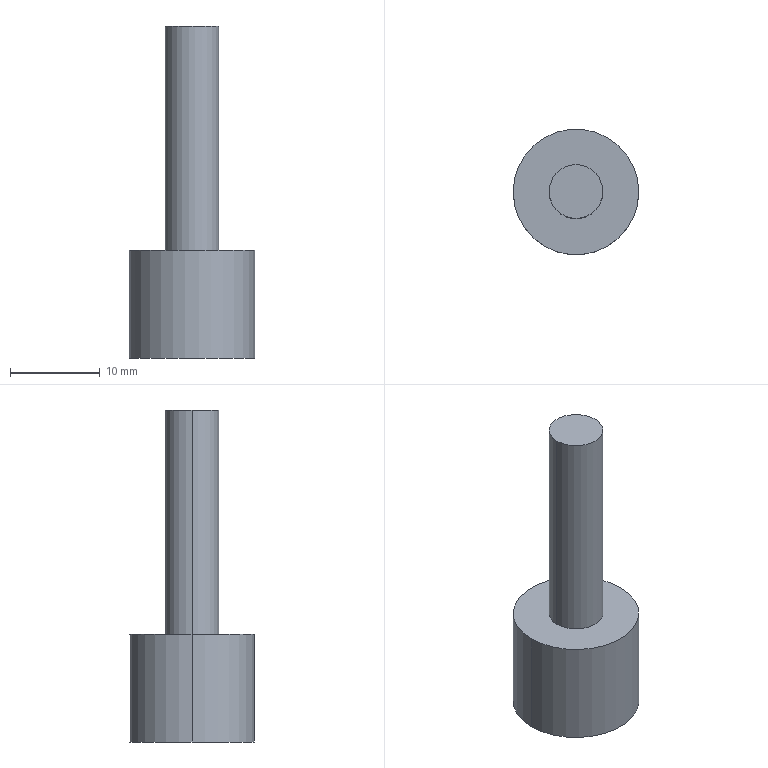Part | SolidWorks | features Extrusion 1, ICE 1 | 1 solid | 7 faces | box 14 x 14 x 37 mm | volume 2554 mm3 | cylinder 4 | plane 3 | commonest cylinder face diameters 6 x2 14 x2
STEP:
#1=CARTESIAN_POINT('',(3.,0.,37.));
#2=VERTEX_POINT('',#1);
#3=CARTESIAN_POINT('',(-3.,0.,37.));
#4=VERTEX_POINT('',#3);
#5=CARTESIAN_POINT('',(0.,0.,37.));
#6=DIRECTION('',(0.,0.,1.));
#7=DIRECTION('',(1.,0.,0.));
#8=AXIS2_PLACEMENT_3D('',#5,#6,#7);
#9=CIRCLE('',#8,3.);
#10=EDGE_CURVE('',#2,#4,#9,.T.);
#11=ORIENTED_EDGE('',*,*,#10,.F.);
#12=CARTESIAN_POINT('',(3.,0.,12.));
#13=VERTEX_POINT('',#12);
#14=CARTESIAN_POINT('',(3.,0.,37.));
#15=DIRECTION('',(0.,0.,-1.));
#16=VECTOR('',#15,1000.);
#17=LINE('',#14,#16);
#18=EDGE_CURVE('',#2,#13,#17,.T.);
#19=ORIENTED_EDGE('',*,*,#18,.T.);
#20=CARTESIAN_POINT('',(-3.,0.,12.));
#21=VERTEX_POINT('',#20);
#22=CARTESIAN_POINT('',(0.,0.,12.));
#23=DIRECTION('',(0.,0.,1.));
#24=DIRECTION('',(1.,0.,0.));
#25=AXIS2_PLACEMENT_3D('',#22,#23,#24);
#26=CIRCLE('',#25,3.);
#27=EDGE_CURVE('',#13,#21,#26,.T.);
#28=ORIENTED_EDGE('',*,*,#27,.T.);
#29=CARTESIAN_POINT('',(-3.,0.,37.));
#30=DIRECTION('',(0.,0.,-1.));
#31=VECTOR('',#30,1000.);
#32=LINE('',#29,#31);
#33=EDGE_CURVE('',#4,#21,#32,.T.);
#34=ORIENTED_EDGE('',*,*,#33,.F.);
#35=EDGE_LOOP('',(#11,#19,#28,#34));
#36=FACE_OUTER_BOUND('',#35,.T.);
#37=CARTESIAN_POINT('',(0.,0.,37.));
#38=DIRECTION('',(0.,0.,-1.));
#39=DIRECTION('',(-1.,0.,0.));
#40=AXIS2_PLACEMENT_3D('',#37,#38,#39);
#41=CYLINDRICAL_SURFACE('',#40,3.);
#42=ADVANCED_FACE('',(#36),#41,.T.);
#43=CARTESIAN_POINT('',(7.,0.,12.));
#44=VERTEX_POINT('',#43);
#45=CARTESIAN_POINT('',(-7.,0.,12.));
#46=VERTEX_POINT('',#45);
#47=CARTESIAN_POINT('',(0.,0.,12.));
#48=DIRECTION('',(0.,0.,1.));
#49=DIRECTION('',(1.,0.,0.));
#50=AXIS2_PLACEMENT_3D('',#47,#48,#49);
#51=CIRCLE('',#50,7.);
#52=EDGE_CURVE('',#44,#46,#51,.T.);
#53=ORIENTED_EDGE('',*,*,#52,.F.);
#54=CARTESIAN_POINT('',(7.,0.,0.));
#55=VERTEX_POINT('',#54);
#56=CARTESIAN_POINT('',(7.,0.,12.));
#57=DIRECTION('',(0.,0.,-1.));
#58=VECTOR('',#57,1000.);
#59=LINE('',#56,#58);
#60=EDGE_CURVE('',#44,#55,#59,.T.);
#61=ORIENTED_EDGE('',*,*,#60,.T.);
#62=CARTESIAN_POINT('',(-7.,0.,0.));
#63=VERTEX_POINT('',#62);
#64=CARTESIAN_POINT('',(0.,0.,0.));
#65=DIRECTION('',(0.,0.,1.));
#66=DIRECTION('',(1.,0.,0.));
#67=AXIS2_PLACEMENT_3D('',#64,#65,#66);
#68=CIRCLE('',#67,7.);
#69=EDGE_CURVE('',#55,#63,#68,.T.);
#70=ORIENTED_EDGE('',*,*,#69,.T.);
#71=CARTESIAN_POINT('',(-7.,0.,12.));
#72=DIRECTION('',(0.,0.,-1.));
#73=VECTOR('',#72,1000.);
#74=LINE('',#71,#73);
#75=EDGE_CURVE('',#46,#63,#74,.T.);
#76=ORIENTED_EDGE('',*,*,#75,.F.);
#77=EDGE_LOOP('',(#53,#61,#70,#76));
#78=FACE_OUTER_BOUND('',#77,.T.);
#79=CARTESIAN_POINT('',(0.,0.,12.));
#80=DIRECTION('',(0.,0.,-1.));
#81=DIRECTION('',(-1.,0.,0.));
#82=AXIS2_PLACEMENT_3D('',#79,#80,#81);
#83=CYLINDRICAL_SURFACE('',#82,7.);
#84=ADVANCED_FACE('',(#78),#83,.T.);
#85=ORIENTED_EDGE('',*,*,#60,.F.);
#86=CARTESIAN_POINT('',(0.,0.,12.));
#87=DIRECTION('',(0.,0.,1.));
#88=DIRECTION('',(1.,0.,0.));
#89=AXIS2_PLACEMENT_3D('',#86,#87,#88);
#90=CIRCLE('',#89,7.);
#91=EDGE_CURVE('',#46,#44,#90,.T.);
#92=ORIENTED_EDGE('',*,*,#91,.F.);
#93=ORIENTED_EDGE('',*,*,#75,.T.);
#94=CARTESIAN_POINT('',(0.,0.,0.));
#95=DIRECTION('',(0.,0.,1.));
#96=DIRECTION('',(1.,0.,0.));
#97=AXIS2_PLACEMENT_3D('',#94,#95,#96);
#98=CIRCLE('',#97,7.);
#99=EDGE_CURVE('',#63,#55,#98,.T.);
#100=ORIENTED_EDGE('',*,*,#99,.T.);
#101=EDGE_LOOP('',(#85,#92,#93,#100));
#102=FACE_OUTER_BOUND('',#101,.T.);
#103=CARTESIAN_POINT('',(0.,0.,12.));
#104=DIRECTION('',(0.,0.,-1.));
#105=DIRECTION('',(-1.,0.,0.));
#106=AXIS2_PLACEMENT_3D('',#103,#104,#105);
#107=CYLINDRICAL_SURFACE('',#106,7.);
#108=ADVANCED_FACE('',(#102),#107,.T.);
#109=CARTESIAN_POINT('',(0.,0.,12.));
#110=DIRECTION('',(0.,0.,1.));
#111=DIRECTION('',(1.,0.,0.));
#112=AXIS2_PLACEMENT_3D('',#109,#110,#111);
#113=CIRCLE('',#112,3.);
#114=EDGE_CURVE('',#21,#13,#113,.T.);
#115=ORIENTED_EDGE('',*,*,#114,.F.);
#116=ORIENTED_EDGE('',*,*,#27,.F.);
#117=EDGE_LOOP('',(#115,#116));
#118=FACE_BOUND('',#117,.T.);
#119=ORIENTED_EDGE('',*,*,#91,.T.);
#120=ORIENTED_EDGE('',*,*,#52,.T.);
#121=EDGE_LOOP('',(#119,#120));
#122=FACE_OUTER_BOUND('',#121,.T.);
#123=CARTESIAN_POINT('',(0.,0.,12.));
#124=DIRECTION('',(0.,0.,1.));
#125=DIRECTION('',(1.,0.,0.));
#126=AXIS2_PLACEMENT_3D('',#123,#124,#125);
#127=PLANE('',#126);
#128=ADVANCED_FACE('',(#118,#122),#127,.T.);
#129=ORIENTED_EDGE('',*,*,#99,.F.);
#130=ORIENTED_EDGE('',*,*,#69,.F.);
#131=EDGE_LOOP('',(#129,#130));
#132=FACE_OUTER_BOUND('',#131,.T.);
#133=CARTESIAN_POINT('',(0.,0.,0.));
#134=DIRECTION('',(0.,0.,1.));
#135=DIRECTION('',(1.,0.,0.));
#136=AXIS2_PLACEMENT_3D('',#133,#134,#135);
#137=PLANE('',#136);
#138=ADVANCED_FACE('',(#132),#137,.F.);
#139=ORIENTED_EDGE('',*,*,#18,.F.);
#140=CARTESIAN_POINT('',(0.,0.,37.));
#141=DIRECTION('',(0.,0.,1.));
#142=DIRECTION('',(1.,0.,0.));
#143=AXIS2_PLACEMENT_3D('',#140,#141,#142);
#144=CIRCLE('',#143,3.);
#145=EDGE_CURVE('',#4,#2,#144,.T.);
#146=ORIENTED_EDGE('',*,*,#145,.F.);
#147=ORIENTED_EDGE('',*,*,#33,.T.);
#148=ORIENTED_EDGE('',*,*,#114,.T.);
#149=EDGE_LOOP('',(#139,#146,#147,#148));
#150=FACE_OUTER_BOUND('',#149,.T.);
#151=CARTESIAN_POINT('',(0.,0.,37.));
#152=DIRECTION('',(0.,0.,-1.));
#153=DIRECTION('',(-1.,0.,0.));
#154=AXIS2_PLACEMENT_3D('',#151,#152,#153);
#155=CYLINDRICAL_SURFACE('',#154,3.);
#156=ADVANCED_FACE('',(#150),#155,.T.);
#157=ORIENTED_EDGE('',*,*,#145,.T.);
#158=ORIENTED_EDGE('',*,*,#10,.T.);
#159=EDGE_LOOP('',(#157,#158));
#160=FACE_OUTER_BOUND('',#159,.T.);
#161=CARTESIAN_POINT('',(0.,0.,37.));
#162=DIRECTION('',(0.,0.,1.));
#163=DIRECTION('',(1.,0.,0.));
#164=AXIS2_PLACEMENT_3D('',#161,#162,#163);
#165=PLANE('',#164);
#166=ADVANCED_FACE('',(#160),#165,.T.);
#167=CLOSED_SHELL('',(#42,#84,#108,#128,#138,#156,#166));
#168=MANIFOLD_SOLID_BREP('',#167);
#169=CARTESIAN_POINT('',(0.,0.,0.));
#170=DIRECTION('',(0.,0.,1.));
#171=DIRECTION('',(1.,0.,0.));
#172=AXIS2_PLACEMENT_3D('',#169,#170,#171);
#173=(LENGTH_UNIT()NAMED_UNIT(*)SI_UNIT(.MILLI.,.METRE.));
#174=UNCERTAINTY_MEASURE_WITH_UNIT(LENGTH_MEASURE(0.00001),#173,'','');
#175=(NAMED_UNIT(*)PLANE_ANGLE_UNIT()SI_UNIT($,.RADIAN.));
#176=(NAMED_UNIT(*)SI_UNIT($,.STERADIAN.)SOLID_ANGLE_UNIT());
#177=(GEOMETRIC_REPRESENTATION_CONTEXT(3)GLOBAL_UNCERTAINTY_ASSIGNED_CONTEXT((#174))GLOBAL_UNIT_ASSIGNED_CONTEXT((#173,#175,#176))REPRESENTATION_CONTEXT('',''));
#178=ADVANCED_BREP_SHAPE_REPRESENTATION('',(#168,#172),#177);